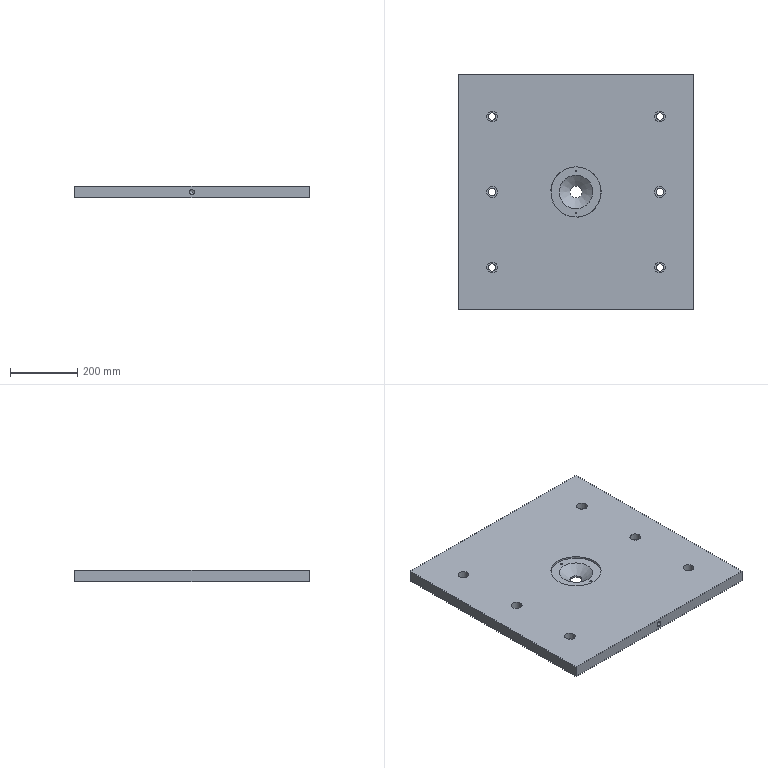Part | NX | features 模具.stp<1>[12] 2 | 1 solid | 55 faces | box 700 x 700 x 35 mm | volume 16813560 mm3 | plane 30 | cylinder 22 | cone 3 | commonest cylinder face diameters 22 x6 32 x6 5 x2 14.1 x2 15.7 x2 16 x2
STEP:
#1=CARTESIAN_POINT('',(-239.,-225.,105.5));
#2=VERTEX_POINT('',#1);
#3=CARTESIAN_POINT('',(-250.,-225.,105.5));
#4=DIRECTION('',(0.,0.,1.));
#5=DIRECTION('',(1.,0.,0.));
#6=AXIS2_PLACEMENT_3D('',#3,#4,#5);
#7=CIRCLE('',#6,11.);
#8=EDGE_CURVE('',#2,#2,#7,.T.);
#9=ORIENTED_EDGE('',*,*,#8,.T.);
#10=EDGE_LOOP('',(#9));
#11=FACE_BOUND('',#10,.T.);
#12=CARTESIAN_POINT('',(-239.,0.,105.5));
#13=VERTEX_POINT('',#12);
#14=CARTESIAN_POINT('',(-250.,0.,105.5));
#15=DIRECTION('',(0.,0.,1.));
#16=DIRECTION('',(1.,0.,0.));
#17=AXIS2_PLACEMENT_3D('',#14,#15,#16);
#18=CIRCLE('',#17,11.);
#19=EDGE_CURVE('',#13,#13,#18,.T.);
#20=ORIENTED_EDGE('',*,*,#19,.T.);
#21=EDGE_LOOP('',(#20));
#22=FACE_BOUND('',#21,.T.);
#23=CARTESIAN_POINT('',(-239.,225.,105.5));
#24=VERTEX_POINT('',#23);
#25=CARTESIAN_POINT('',(-250.,225.,105.5));
#26=DIRECTION('',(0.,0.,1.));
#27=DIRECTION('',(1.,0.,0.));
#28=AXIS2_PLACEMENT_3D('',#25,#26,#27);
#29=CIRCLE('',#28,11.);
#30=EDGE_CURVE('',#24,#24,#29,.T.);
#31=ORIENTED_EDGE('',*,*,#30,.T.);
#32=EDGE_LOOP('',(#31));
#33=FACE_BOUND('',#32,.T.);
#34=CARTESIAN_POINT('',(261.,225.,105.5));
#35=VERTEX_POINT('',#34);
#36=CARTESIAN_POINT('',(250.,225.,105.5));
#37=DIRECTION('',(0.,0.,1.));
#38=DIRECTION('',(1.,0.,0.));
#39=AXIS2_PLACEMENT_3D('',#36,#37,#38);
#40=CIRCLE('',#39,11.);
#41=EDGE_CURVE('',#35,#35,#40,.T.);
#42=ORIENTED_EDGE('',*,*,#41,.T.);
#43=EDGE_LOOP('',(#42));
#44=FACE_BOUND('',#43,.T.);
#45=CARTESIAN_POINT('',(261.,0.,105.5));
#46=VERTEX_POINT('',#45);
#47=CARTESIAN_POINT('',(250.,0.,105.5));
#48=DIRECTION('',(0.,0.,1.));
#49=DIRECTION('',(1.,0.,0.));
#50=AXIS2_PLACEMENT_3D('',#47,#48,#49);
#51=CIRCLE('',#50,11.);
#52=EDGE_CURVE('',#46,#46,#51,.T.);
#53=ORIENTED_EDGE('',*,*,#52,.T.);
#54=EDGE_LOOP('',(#53));
#55=FACE_BOUND('',#54,.T.);
#56=CARTESIAN_POINT('',(261.,-225.,105.5));
#57=VERTEX_POINT('',#56);
#58=CARTESIAN_POINT('',(250.,-225.,105.5));
#59=DIRECTION('',(0.,0.,1.));
#60=DIRECTION('',(1.,0.,0.));
#61=AXIS2_PLACEMENT_3D('',#58,#59,#60);
#62=CIRCLE('',#61,11.);
#63=EDGE_CURVE('',#57,#57,#62,.T.);
#64=ORIENTED_EDGE('',*,*,#63,.T.);
#65=EDGE_LOOP('',(#64));
#66=FACE_BOUND('',#65,.T.);
#67=CARTESIAN_POINT('',(350.,-350.,105.5));
#68=VERTEX_POINT('',#67);
#69=CARTESIAN_POINT('',(350.,350.,105.5));
#70=VERTEX_POINT('',#69);
#71=CARTESIAN_POINT('',(350.,0.,105.5));
#72=DIRECTION('',(0.,1.,0.));
#73=VECTOR('',#72,1000.);
#74=LINE('',#71,#73);
#75=EDGE_CURVE('',#68,#70,#74,.T.);
#76=ORIENTED_EDGE('',*,*,#75,.F.);
#77=CARTESIAN_POINT('',(-350.,-350.,105.5));
#78=VERTEX_POINT('',#77);
#79=CARTESIAN_POINT('',(0.,-350.,105.5));
#80=DIRECTION('',(1.,0.,0.));
#81=VECTOR('',#80,1000.);
#82=LINE('',#79,#81);
#83=EDGE_CURVE('',#78,#68,#82,.T.);
#84=ORIENTED_EDGE('',*,*,#83,.F.);
#85=CARTESIAN_POINT('',(-350.,350.,105.5));
#86=VERTEX_POINT('',#85);
#87=CARTESIAN_POINT('',(-350.,0.,105.5));
#88=DIRECTION('',(0.,-1.,0.));
#89=VECTOR('',#88,1000.);
#90=LINE('',#87,#89);
#91=EDGE_CURVE('',#86,#78,#90,.T.);
#92=ORIENTED_EDGE('',*,*,#91,.F.);
#93=CARTESIAN_POINT('',(0.,350.,105.5));
#94=DIRECTION('',(-1.,0.,0.));
#95=VECTOR('',#94,1000.);
#96=LINE('',#93,#95);
#97=EDGE_CURVE('',#70,#86,#96,.T.);
#98=ORIENTED_EDGE('',*,*,#97,.F.);
#99=EDGE_LOOP('',(#76,#84,#92,#98));
#100=FACE_BOUND('',#99,.T.);
#101=CARTESIAN_POINT('',(312.,-319.,105.5));
#102=VERTEX_POINT('',#101);
#103=CARTESIAN_POINT('',(312.,-322.,105.5));
#104=VERTEX_POINT('',#103);
#105=CARTESIAN_POINT('',(312.,-322.,105.5));
#106=DIRECTION('',(0.,-1.,0.));
#107=VECTOR('',#106,1000.);
#108=LINE('',#105,#107);
#109=EDGE_CURVE('',#102,#104,#108,.T.);
#110=ORIENTED_EDGE('',*,*,#109,.T.);
#111=CARTESIAN_POINT('',(322.,-322.,105.5));
#112=VERTEX_POINT('',#111);
#113=CARTESIAN_POINT('',(312.,-322.,105.5));
#114=DIRECTION('',(1.,0.,0.));
#115=VECTOR('',#114,1000.);
#116=LINE('',#113,#115);
#117=EDGE_CURVE('',#104,#112,#116,.T.);
#118=ORIENTED_EDGE('',*,*,#117,.T.);
#119=CARTESIAN_POINT('',(322.,-312.,105.5));
#120=VERTEX_POINT('',#119);
#121=CARTESIAN_POINT('',(322.,-312.,105.5));
#122=DIRECTION('',(0.,1.,0.));
#123=VECTOR('',#122,1000.);
#124=LINE('',#121,#123);
#125=EDGE_CURVE('',#112,#120,#124,.T.);
#126=ORIENTED_EDGE('',*,*,#125,.T.);
#127=CARTESIAN_POINT('',(319.,-312.,105.5));
#128=VERTEX_POINT('',#127);
#129=CARTESIAN_POINT('',(319.,-312.,105.5));
#130=DIRECTION('',(-1.,0.,0.));
#131=VECTOR('',#130,1000.);
#132=LINE('',#129,#131);
#133=EDGE_CURVE('',#120,#128,#132,.T.);
#134=ORIENTED_EDGE('',*,*,#133,.T.);
#135=CARTESIAN_POINT('',(319.,-319.,105.5));
#136=VERTEX_POINT('',#135);
#137=CARTESIAN_POINT('',(319.,-319.,105.5));
#138=DIRECTION('',(0.,-1.,0.));
#139=VECTOR('',#138,1000.);
#140=LINE('',#137,#139);
#141=EDGE_CURVE('',#128,#136,#140,.T.);
#142=ORIENTED_EDGE('',*,*,#141,.T.);
#143=CARTESIAN_POINT('',(312.,-319.,105.5));
#144=DIRECTION('',(-1.,0.,0.));
#145=VECTOR('',#144,1000.);
#146=LINE('',#143,#145);
#147=EDGE_CURVE('',#136,#102,#146,.T.);
#148=ORIENTED_EDGE('',*,*,#147,.T.);
#149=EDGE_LOOP('',(#110,#118,#126,#134,#142,#148));
#150=FACE_BOUND('',#149,.T.);
#151=CARTESIAN_POINT('',(-18.,0.,105.5));
#152=VERTEX_POINT('',#151);
#153=CARTESIAN_POINT('',(0.,0.,105.5));
#154=DIRECTION('',(0.,0.,-1.));
#155=DIRECTION('',(-1.,0.,0.));
#156=AXIS2_PLACEMENT_3D('',#153,#154,#155);
#157=CIRCLE('',#156,18.);
#158=EDGE_CURVE('',#152,#152,#157,.T.);
#159=ORIENTED_EDGE('',*,*,#158,.F.);
#160=EDGE_LOOP('',(#159));
#161=FACE_BOUND('',#160,.T.);
#162=CARTESIAN_POINT('',(0.,0.,105.5));
#163=DIRECTION('',(0.,0.,-1.));
#164=DIRECTION('',(0.,-1.,0.));
#165=AXIS2_PLACEMENT_3D('',#162,#163,#164);
#166=PLANE('',#165);
#167=ADVANCED_FACE('',(#11,#22,#33,#44,#55,#66,#100,#150,#161),#166,.T.);
#168=CARTESIAN_POINT('',(-18.,0.,110.5));
#169=VERTEX_POINT('',#168);
#170=CARTESIAN_POINT('',(0.,0.,110.5));
#171=DIRECTION('',(0.,0.,1.));
#172=DIRECTION('',(-1.,0.,0.));
#173=AXIS2_PLACEMENT_3D('',#170,#171,#172);
#174=CIRCLE('',#173,18.);
#175=EDGE_CURVE('',#169,#169,#174,.T.);
#176=ORIENTED_EDGE('',*,*,#175,.T.);
#177=EDGE_LOOP('',(#176));
#178=FACE_BOUND('',#177,.T.);
#179=ORIENTED_EDGE('',*,*,#158,.T.);
#180=EDGE_LOOP('',(#179));
#181=FACE_BOUND('',#180,.T.);
#182=CARTESIAN_POINT('',(0.,0.,105.));
#183=DIRECTION('',(0.,0.,1.));
#184=DIRECTION('',(1.,0.,0.));
#185=AXIS2_PLACEMENT_3D('',#182,#183,#184);
#186=CYLINDRICAL_SURFACE('',#185,18.);
#187=ADVANCED_FACE('',(#178,#181),#186,.F.);
#188=ORIENTED_EDGE('',*,*,#109,.F.);
#189=CARTESIAN_POINT('',(312.,-319.,105.8));
#190=VERTEX_POINT('',#189);
#191=CARTESIAN_POINT('',(312.,-319.,105.8));
#192=DIRECTION('',(0.,0.,-1.));
#193=VECTOR('',#192,1000.);
#194=LINE('',#191,#193);
#195=EDGE_CURVE('',#190,#102,#194,.T.);
#196=ORIENTED_EDGE('',*,*,#195,.F.);
#197=CARTESIAN_POINT('',(312.,-322.,105.8));
#198=VERTEX_POINT('',#197);
#199=CARTESIAN_POINT('',(312.,-322.,105.8));
#200=DIRECTION('',(0.,-1.,0.));
#201=VECTOR('',#200,1000.);
#202=LINE('',#199,#201);
#203=EDGE_CURVE('',#190,#198,#202,.T.);
#204=ORIENTED_EDGE('',*,*,#203,.T.);
#205=CARTESIAN_POINT('',(312.,-322.,105.8));
#206=DIRECTION('',(0.,0.,-1.));
#207=VECTOR('',#206,1000.);
#208=LINE('',#205,#207);
#209=EDGE_CURVE('',#198,#104,#208,.T.);
#210=ORIENTED_EDGE('',*,*,#209,.T.);
#211=EDGE_LOOP('',(#188,#196,#204,#210));
#212=FACE_BOUND('',#211,.T.);
#213=CARTESIAN_POINT('',(312.,-322.,105.8));
#214=DIRECTION('',(1.,0.,0.));
#215=DIRECTION('',(0.,1.,0.));
#216=AXIS2_PLACEMENT_3D('',#213,#214,#215);
#217=PLANE('',#216);
#218=ADVANCED_FACE('',(#212),#217,.T.);
#219=ORIENTED_EDGE('',*,*,#117,.F.);
#220=ORIENTED_EDGE('',*,*,#209,.F.);
#221=CARTESIAN_POINT('',(322.,-322.,105.8));
#222=VERTEX_POINT('',#221);
#223=CARTESIAN_POINT('',(312.,-322.,105.8));
#224=DIRECTION('',(1.,0.,0.));
#225=VECTOR('',#224,1000.);
#226=LINE('',#223,#225);
#227=EDGE_CURVE('',#198,#222,#226,.T.);
#228=ORIENTED_EDGE('',*,*,#227,.T.);
#229=CARTESIAN_POINT('',(322.,-322.,105.8));
#230=DIRECTION('',(0.,0.,-1.));
#231=VECTOR('',#230,1000.);
#232=LINE('',#229,#231);
#233=EDGE_CURVE('',#222,#112,#232,.T.);
#234=ORIENTED_EDGE('',*,*,#233,.T.);
#235=EDGE_LOOP('',(#219,#220,#228,#234));
#236=FACE_BOUND('',#235,.T.);
#237=CARTESIAN_POINT('',(312.,-322.,105.8));
#238=DIRECTION('',(0.,1.,0.));
#239=DIRECTION('',(1.,0.,0.));
#240=AXIS2_PLACEMENT_3D('',#237,#238,#239);
#241=PLANE('',#240);
#242=ADVANCED_FACE('',(#236),#241,.T.);
#243=ORIENTED_EDGE('',*,*,#125,.F.);
#244=ORIENTED_EDGE('',*,*,#233,.F.);
#245=CARTESIAN_POINT('',(322.,-312.,105.8));
#246=VERTEX_POINT('',#245);
#247=CARTESIAN_POINT('',(322.,-312.,105.8));
#248=DIRECTION('',(0.,1.,0.));
#249=VECTOR('',#248,1000.);
#250=LINE('',#247,#249);
#251=EDGE_CURVE('',#222,#246,#250,.T.);
#252=ORIENTED_EDGE('',*,*,#251,.T.);
#253=CARTESIAN_POINT('',(322.,-312.,105.8));
#254=DIRECTION('',(0.,0.,-1.));
#255=VECTOR('',#254,1000.);
#256=LINE('',#253,#255);
#257=EDGE_CURVE('',#246,#120,#256,.T.);
#258=ORIENTED_EDGE('',*,*,#257,.T.);
#259=EDGE_LOOP('',(#243,#244,#252,#258));
#260=FACE_BOUND('',#259,.T.);
#261=CARTESIAN_POINT('',(322.,-312.,105.8));
#262=DIRECTION('',(-1.,0.,0.));
#263=DIRECTION('',(0.,0.,1.));
#264=AXIS2_PLACEMENT_3D('',#261,#262,#263);
#265=PLANE('',#264);
#266=ADVANCED_FACE('',(#260),#265,.T.);
#267=ORIENTED_EDGE('',*,*,#133,.F.);
#268=ORIENTED_EDGE('',*,*,#257,.F.);
#269=CARTESIAN_POINT('',(319.,-312.,105.8));
#270=VERTEX_POINT('',#269);
#271=CARTESIAN_POINT('',(319.,-312.,105.8));
#272=DIRECTION('',(-1.,0.,0.));
#273=VECTOR('',#272,1000.);
#274=LINE('',#271,#273);
#275=EDGE_CURVE('',#246,#270,#274,.T.);
#276=ORIENTED_EDGE('',*,*,#275,.T.);
#277=CARTESIAN_POINT('',(319.,-312.,105.8));
#278=DIRECTION('',(0.,0.,-1.));
#279=VECTOR('',#278,1000.);
#280=LINE('',#277,#279);
#281=EDGE_CURVE('',#270,#128,#280,.T.);
#282=ORIENTED_EDGE('',*,*,#281,.T.);
#283=EDGE_LOOP('',(#267,#268,#276,#282));
#284=FACE_BOUND('',#283,.T.);
#285=CARTESIAN_POINT('',(319.,-312.,105.8));
#286=DIRECTION('',(0.,-1.,0.));
#287=DIRECTION('',(0.,0.,-1.));
#288=AXIS2_PLACEMENT_3D('',#285,#286,#287);
#289=PLANE('',#288);
#290=ADVANCED_FACE('',(#284),#289,.T.);
#291=ORIENTED_EDGE('',*,*,#141,.F.);
#292=ORIENTED_EDGE('',*,*,#281,.F.);
#293=CARTESIAN_POINT('',(319.,-319.,105.8));
#294=VERTEX_POINT('',#293);
#295=CARTESIAN_POINT('',(319.,-319.,105.8));
#296=DIRECTION('',(0.,-1.,0.));
#297=VECTOR('',#296,1000.);
#298=LINE('',#295,#297);
#299=EDGE_CURVE('',#270,#294,#298,.T.);
#300=ORIENTED_EDGE('',*,*,#299,.T.);
#301=CARTESIAN_POINT('',(319.,-319.,105.8));
#302=DIRECTION('',(0.,0.,-1.));
#303=VECTOR('',#302,1000.);
#304=LINE('',#301,#303);
#305=EDGE_CURVE('',#294,#136,#304,.T.);
#306=ORIENTED_EDGE('',*,*,#305,.T.);
#307=EDGE_LOOP('',(#291,#292,#300,#306));
#308=FACE_BOUND('',#307,.T.);
#309=CARTESIAN_POINT('',(319.,-319.,105.8));
#310=DIRECTION('',(1.,0.,0.));
#311=DIRECTION('',(0.,1.,0.));
#312=AXIS2_PLACEMENT_3D('',#309,#310,#311);
#313=PLANE('',#312);
#314=ADVANCED_FACE('',(#308),#313,.T.);
#315=ORIENTED_EDGE('',*,*,#147,.F.);
#316=ORIENTED_EDGE('',*,*,#305,.F.);
#317=CARTESIAN_POINT('',(312.,-319.,105.8));
#318=DIRECTION('',(-1.,0.,0.));
#319=VECTOR('',#318,1000.);
#320=LINE('',#317,#319);
#321=EDGE_CURVE('',#294,#190,#320,.T.);
#322=ORIENTED_EDGE('',*,*,#321,.T.);
#323=ORIENTED_EDGE('',*,*,#195,.T.);
#324=EDGE_LOOP('',(#315,#316,#322,#323));
#325=FACE_BOUND('',#324,.T.);
#326=CARTESIAN_POINT('',(312.,-319.,105.8));
#327=DIRECTION('',(0.,-1.,0.));
#328=DIRECTION('',(0.,0.,-1.));
#329=AXIS2_PLACEMENT_3D('',#326,#327,#328);
#330=PLANE('',#329);
#331=ADVANCED_FACE('',(#325),#330,.T.);
#332=ORIENTED_EDGE('',*,*,#227,.F.);
#333=ORIENTED_EDGE('',*,*,#203,.F.);
#334=ORIENTED_EDGE('',*,*,#321,.F.);
#335=ORIENTED_EDGE('',*,*,#299,.F.);
#336=ORIENTED_EDGE('',*,*,#275,.F.);
#337=ORIENTED_EDGE('',*,*,#251,.F.);
#338=EDGE_LOOP('',(#332,#333,#334,#335,#336,#337));
#339=FACE_BOUND('',#338,.T.);
#340=CARTESIAN_POINT('',(322.,-322.,105.8));
#341=DIRECTION('',(0.,0.,1.));
#342=DIRECTION('',(1.,0.,0.));
#343=AXIS2_PLACEMENT_3D('',#340,#341,#342);
#344=PLANE('',#343);
#345=ADVANCED_FACE('',(#339),#344,.F.);
#346=CARTESIAN_POINT('',(0.,65.,122.5));
#347=VERTEX_POINT('',#346);
#348=CARTESIAN_POINT('',(0.,62.5,122.5));
#349=DIRECTION('',(0.,0.,-1.));
#350=DIRECTION('',(0.,1.,0.));
#351=AXIS2_PLACEMENT_3D('',#348,#349,#350);
#352=CIRCLE('',#351,2.5);
#353=EDGE_CURVE('',#347,#347,#352,.T.);
#354=ORIENTED_EDGE('',*,*,#353,.F.);
#355=EDGE_LOOP('',(#354));
#356=FACE_BOUND('',#355,.T.);
#357=CARTESIAN_POINT('',(0.,62.5,122.5));
#358=DIRECTION('',(0.,0.,-1.));
#359=DIRECTION('',(-1.,0.,0.));
#360=AXIS2_PLACEMENT_3D('',#357,#358,#359);
#361=PLANE('',#360);
#362=ADVANCED_FACE('',(#356),#361,.F.);
#363=CARTESIAN_POINT('',(0.,65.,135.5));
#364=VERTEX_POINT('',#363);
#365=CARTESIAN_POINT('',(0.,62.5,135.5));
#366=DIRECTION('',(0.,0.,-1.));
#367=DIRECTION('',(0.,1.,0.));
#368=AXIS2_PLACEMENT_3D('',#365,#366,#367);
#369=CIRCLE('',#368,2.5);
#370=EDGE_CURVE('',#364,#364,#369,.T.);
#371=ORIENTED_EDGE('',*,*,#370,.F.);
#372=EDGE_LOOP('',(#371));
#373=FACE_BOUND('',#372,.T.);
#374=ORIENTED_EDGE('',*,*,#353,.T.);
#375=EDGE_LOOP('',(#374));
#376=FACE_BOUND('',#375,.T.);
#377=CARTESIAN_POINT('',(0.,62.5,127.5));
#378=DIRECTION('',(0.,0.,1.));
#379=DIRECTION('',(1.,0.,0.));
#380=AXIS2_PLACEMENT_3D('',#377,#378,#379);
#381=CYLINDRICAL_SURFACE('',#380,2.5);
#382=ADVANCED_FACE('',(#373,#376),#381,.F.);
#383=CARTESIAN_POINT('',(0.,-60.,122.5));
#384=VERTEX_POINT('',#383);
#385=CARTESIAN_POINT('',(0.,-62.5,122.5));
#386=DIRECTION('',(0.,0.,-1.));
#387=DIRECTION('',(0.,1.,0.));
#388=AXIS2_PLACEMENT_3D('',#385,#386,#387);
#389=CIRCLE('',#388,2.5);
#390=EDGE_CURVE('',#384,#384,#389,.T.);
#391=ORIENTED_EDGE('',*,*,#390,.F.);
#392=EDGE_LOOP('',(#391));
#393=FACE_BOUND('',#392,.T.);
#394=CARTESIAN_POINT('',(0.,-62.5,122.5));
#395=DIRECTION('',(0.,0.,-1.));
#396=DIRECTION('',(-1.,0.,0.));
#397=AXIS2_PLACEMENT_3D('',#394,#395,#396);
#398=PLANE('',#397);
#399=ADVANCED_FACE('',(#393),#398,.F.);
#400=CARTESIAN_POINT('',(0.,-60.,135.5));
#401=VERTEX_POINT('',#400);
#402=CARTESIAN_POINT('',(0.,-62.5,135.5));
#403=DIRECTION('',(0.,0.,-1.));
#404=DIRECTION('',(0.,1.,0.));
#405=AXIS2_PLACEMENT_3D('',#402,#403,#404);
#406=CIRCLE('',#405,2.5);
#407=EDGE_CURVE('',#401,#401,#406,.T.);
#408=ORIENTED_EDGE('',*,*,#407,.F.);
#409=EDGE_LOOP('',(#408));
#410=FACE_BOUND('',#409,.T.);
#411=ORIENTED_EDGE('',*,*,#390,.T.);
#412=EDGE_LOOP('',(#411));
#413=FACE_BOUND('',#412,.T.);
#414=CARTESIAN_POINT('',(0.,-62.5,127.5));
#415=DIRECTION('',(0.,0.,1.));
#416=DIRECTION('',(1.,0.,0.));
#417=AXIS2_PLACEMENT_3D('',#414,#415,#416);
#418=CYLINDRICAL_SURFACE('',#417,2.5);
#419=ADVANCED_FACE('',(#410,#413),#418,.F.);
#420=CARTESIAN_POINT('',(0.,75.,135.5));
#421=VERTEX_POINT('',#420);
#422=CARTESIAN_POINT('',(0.,0.,135.5));
#423=DIRECTION('',(0.,0.,-1.));
#424=DIRECTION('',(0.,1.,0.));
#425=AXIS2_PLACEMENT_3D('',#422,#423,#424);
#426=CIRCLE('',#425,75.);
#427=EDGE_CURVE('',#421,#421,#426,.T.);
#428=ORIENTED_EDGE('',*,*,#427,.T.);
#429=EDGE_LOOP('',(#428));
#430=FACE_BOUND('',#429,.T.);
#431=CARTESIAN_POINT('',(75.,0.,140.5));
#432=VERTEX_POINT('',#431);
#433=CARTESIAN_POINT('',(0.,0.,140.5));
#434=DIRECTION('',(0.,0.,1.));
#435=DIRECTION('',(1.,0.,0.));
#436=AXIS2_PLACEMENT_3D('',#433,#434,#435);
#437=CIRCLE('',#436,75.);
#438=EDGE_CURVE('',#432,#432,#437,.T.);
#439=ORIENTED_EDGE('',*,*,#438,.T.);
#440=EDGE_LOOP('',(#439));
#441=FACE_BOUND('',#440,.T.);
#442=CARTESIAN_POINT('',(0.,0.,150.5));
#443=DIRECTION('',(0.,0.,-1.));
#444=DIRECTION('',(0.,1.,0.));
#445=AXIS2_PLACEMENT_3D('',#442,#443,#444);
#446=CYLINDRICAL_SURFACE('',#445,75.);
#447=ADVANCED_FACE('',(#430,#441),#446,.F.);
#448=CARTESIAN_POINT('',(0.,49.999,135.5));
#449=VERTEX_POINT('',#448);
#450=CARTESIAN_POINT('',(0.,0.,135.5));
#451=DIRECTION('',(0.,0.,1.));
#452=DIRECTION('',(0.,1.,0.));
#453=AXIS2_PLACEMENT_3D('',#450,#451,#452);
#454=CIRCLE('',#453,49.999);
#455=EDGE_CURVE('',#449,#449,#454,.T.);
#456=ORIENTED_EDGE('',*,*,#455,.F.);
#457=EDGE_LOOP('',(#456));
#458=FACE_BOUND('',#457,.T.);
#459=ORIENTED_EDGE('',*,*,#427,.F.);
#460=EDGE_LOOP('',(#459));
#461=FACE_BOUND('',#460,.T.);
#462=ORIENTED_EDGE('',*,*,#407,.T.);
#463=EDGE_LOOP('',(#462));
#464=FACE_BOUND('',#463,.T.);
#465=ORIENTED_EDGE('',*,*,#370,.T.);
#466=EDGE_LOOP('',(#465));
#467=FACE_BOUND('',#466,.T.);
#468=CARTESIAN_POINT('',(0.,0.,135.5));
#469=DIRECTION('',(0.,0.,-1.));
#470=DIRECTION('',(-1.,0.,0.));
#471=AXIS2_PLACEMENT_3D('',#468,#469,#470);
#472=PLANE('',#471);
#473=ADVANCED_FACE('',(#458,#461,#464,#467),#472,.F.);
#474=CARTESIAN_POINT('',(-234.,-225.,119.5));
#475=VERTEX_POINT('',#474);
#476=CARTESIAN_POINT('',(-250.,-225.,119.5));
#477=DIRECTION('',(0.,0.,1.));
#478=DIRECTION('',(1.,0.,0.));
#479=AXIS2_PLACEMENT_3D('',#476,#477,#478);
#480=CIRCLE('',#479,16.);
#481=EDGE_CURVE('',#475,#475,#480,.T.);
#482=ORIENTED_EDGE('',*,*,#481,.F.);
#483=EDGE_LOOP('',(#482));
#484=FACE_BOUND('',#483,.T.);
#485=CARTESIAN_POINT('',(-234.,-225.,140.5));
#486=VERTEX_POINT('',#485);
#487=CARTESIAN_POINT('',(-250.,-225.,140.5));
#488=DIRECTION('',(0.,0.,-1.));
#489=DIRECTION('',(1.,0.,0.));
#490=AXIS2_PLACEMENT_3D('',#487,#488,#489);
#491=CIRCLE('',#490,16.);
#492=EDGE_CURVE('',#486,#486,#491,.T.);
#493=ORIENTED_EDGE('',*,*,#492,.F.);
#494=EDGE_LOOP('',(#493));
#495=FACE_BOUND('',#494,.T.);
#496=CARTESIAN_POINT('',(-250.,-225.,119.5));
#497=DIRECTION('',(0.,0.,1.));
#498=DIRECTION('',(1.,0.,0.));
#499=AXIS2_PLACEMENT_3D('',#496,#497,#498);
#500=CYLINDRICAL_SURFACE('',#499,16.);
#501=ADVANCED_FACE('',(#484,#495),#500,.F.);
#502=ORIENTED_EDGE('',*,*,#481,.T.);
#503=EDGE_LOOP('',(#502));
#504=FACE_BOUND('',#503,.T.);
#505=CARTESIAN_POINT('',(-261.,-225.,119.5));
#506=VERTEX_POINT('',#505);
#507=CARTESIAN_POINT('',(-250.,-225.,119.5));
#508=DIRECTION('',(0.,0.,1.));
#509=DIRECTION('',(-1.,0.,0.));
#510=AXIS2_PLACEMENT_3D('',#507,#508,#509);
#511=CIRCLE('',#510,11.);
#512=EDGE_CURVE('',#506,#506,#511,.T.);
#513=ORIENTED_EDGE('',*,*,#512,.F.);
#514=EDGE_LOOP('',(#513));
#515=FACE_BOUND('',#514,.T.);
#516=CARTESIAN_POINT('',(-250.,-225.,119.5));
#517=DIRECTION('',(0.,0.,-1.));
#518=DIRECTION('',(0.,-1.,0.));
#519=AXIS2_PLACEMENT_3D('',#516,#517,#518);
#520=PLANE('',#519);
#521=ADVANCED_FACE('',(#504,#515),#520,.F.);
#522=CARTESIAN_POINT('',(-234.,0.,119.5));
#523=VERTEX_POINT('',#522);
#524=CARTESIAN_POINT('',(-250.,0.,119.5));
#525=DIRECTION('',(0.,0.,1.));
#526=DIRECTION('',(1.,0.,0.));
#527=AXIS2_PLACEMENT_3D('',#524,#525,#526);
#528=CIRCLE('',#527,16.);
#529=EDGE_CURVE('',#523,#523,#528,.T.);
#530=ORIENTED_EDGE('',*,*,#529,.F.);
#531=EDGE_LOOP('',(#530));
#532=FACE_BOUND('',#531,.T.);
#533=CARTESIAN_POINT('',(-234.,0.,140.5));
#534=VERTEX_POINT('',#533);
#535=CARTESIAN_POINT('',(-250.,0.,140.5));
#536=DIRECTION('',(0.,0.,-1.));
#537=DIRECTION('',(1.,0.,0.));
#538=AXIS2_PLACEMENT_3D('',#535,#536,#537);
#539=CIRCLE('',#538,16.);
#540=EDGE_CURVE('',#534,#534,#539,.T.);
#541=ORIENTED_EDGE('',*,*,#540,.F.);
#542=EDGE_LOOP('',(#541));
#543=FACE_BOUND('',#542,.T.);
#544=CARTESIAN_POINT('',(-250.,0.,119.5));
#545=DIRECTION('',(0.,0.,1.));
#546=DIRECTION('',(1.,0.,0.));
#547=AXIS2_PLACEMENT_3D('',#544,#545,#546);
#548=CYLINDRICAL_SURFACE('',#547,16.);
#549=ADVANCED_FACE('',(#532,#543),#548,.F.);
#550=ORIENTED_EDGE('',*,*,#529,.T.);
#551=EDGE_LOOP('',(#550));
#552=FACE_BOUND('',#551,.T.);
#553=CARTESIAN_POINT('',(-261.,0.,119.5));
#554=VERTEX_POINT('',#553);
#555=CARTESIAN_POINT('',(-250.,0.,119.5));
#556=DIRECTION('',(0.,0.,1.));
#557=DIRECTION('',(-1.,0.,0.));
#558=AXIS2_PLACEMENT_3D('',#555,#556,#557);
#559=CIRCLE('',#558,11.);
#560=EDGE_CURVE('',#554,#554,#559,.T.);
#561=ORIENTED_EDGE('',*,*,#560,.F.);
#562=EDGE_LOOP('',(#561));
#563=FACE_BOUND('',#562,.T.);
#564=CARTESIAN_POINT('',(-250.,0.,119.5));
#565=DIRECTION('',(0.,0.,-1.));
#566=DIRECTION('',(0.,-1.,0.));
#567=AXIS2_PLACEMENT_3D('',#564,#565,#566);
#568=PLANE('',#567);
#569=ADVANCED_FACE('',(#552,#563),#568,.F.);
#570=CARTESIAN_POINT('',(-234.,225.,119.5));
#571=VERTEX_POINT('',#570);
#572=CARTESIAN_POINT('',(-250.,225.,119.5));
#573=DIRECTION('',(0.,0.,1.));
#574=DIRECTION('',(1.,0.,0.));
#575=AXIS2_PLACEMENT_3D('',#572,#573,#574);
#576=CIRCLE('',#575,16.);
#577=EDGE_CURVE('',#571,#571,#576,.T.);
#578=ORIENTED_EDGE('',*,*,#577,.F.);
#579=EDGE_LOOP('',(#578));
#580=FACE_BOUND('',#579,.T.);
#581=CARTESIAN_POINT('',(-234.,225.,140.5));
#582=VERTEX_POINT('',#581);
#583=CARTESIAN_POINT('',(-250.,225.,140.5));
#584=DIRECTION('',(0.,0.,-1.));
#585=DIRECTION('',(1.,0.,0.));
#586=AXIS2_PLACEMENT_3D('',#583,#584,#585);
#587=CIRCLE('',#586,16.);
#588=EDGE_CURVE('',#582,#582,#587,.T.);
#589=ORIENTED_EDGE('',*,*,#588,.F.);
#590=EDGE_LOOP('',(#589));
#591=FACE_BOUND('',#590,.T.);
#592=CARTESIAN_POINT('',(-250.,225.,119.5));
#593=DIRECTION('',(0.,0.,1.));
#594=DIRECTION('',(1.,0.,0.));
#595=AXIS2_PLACEMENT_3D('',#592,#593,#594);
#596=CYLINDRICAL_SURFACE('',#595,16.);
#597=ADVANCED_FACE('',(#580,#591),#596,.F.);
#598=ORIENTED_EDGE('',*,*,#577,.T.);
#599=EDGE_LOOP('',(#598));
#600=FACE_BOUND('',#599,.T.);
#601=CARTESIAN_POINT('',(-261.,225.,119.5));
#602=VERTEX_POINT('',#601);
#603=CARTESIAN_POINT('',(-250.,225.,119.5));
#604=DIRECTION('',(0.,0.,1.));
#605=DIRECTION('',(-1.,0.,0.));
#606=AXIS2_PLACEMENT_3D('',#603,#604,#605);
#607=CIRCLE('',#606,11.);
#608=EDGE_CURVE('',#602,#602,#607,.T.);
#609=ORIENTED_EDGE('',*,*,#608,.F.);
#610=EDGE_LOOP('',(#609));
#611=FACE_BOUND('',#610,.T.);
#612=CARTESIAN_POINT('',(-250.,225.,119.5));
#613=DIRECTION('',(0.,0.,-1.));
#614=DIRECTION('',(0.,-1.,0.));
#615=AXIS2_PLACEMENT_3D('',#612,#613,#614);
#616=PLANE('',#615);
#617=ADVANCED_FACE('',(#600,#611),#616,.F.);
#618=CARTESIAN_POINT('',(266.,225.,119.5));
#619=VERTEX_POINT('',#618);
#620=CARTESIAN_POINT('',(250.,225.,119.5));
#621=DIRECTION('',(0.,0.,1.));
#622=DIRECTION('',(1.,0.,0.));
#623=AXIS2_PLACEMENT_3D('',#620,#621,#622);
#624=CIRCLE('',#623,16.);
#625=EDGE_CURVE('',#619,#619,#624,.T.);
#626=ORIENTED_EDGE('',*,*,#625,.F.);
#627=EDGE_LOOP('',(#626));
#628=FACE_BOUND('',#627,.T.);
#629=CARTESIAN_POINT('',(266.,225.,140.5));
#630=VERTEX_POINT('',#629);
#631=CARTESIAN_POINT('',(250.,225.,140.5));
#632=DIRECTION('',(0.,0.,-1.));
#633=DIRECTION('',(1.,0.,0.));
#634=AXIS2_PLACEMENT_3D('',#631,#632,#633);
#635=CIRCLE('',#634,16.);
#636=EDGE_CURVE('',#630,#630,#635,.T.);
#637=ORIENTED_EDGE('',*,*,#636,.F.);
#638=EDGE_LOOP('',(#637));
#639=FACE_BOUND('',#638,.T.);
#640=CARTESIAN_POINT('',(250.,225.,119.5));
#641=DIRECTION('',(0.,0.,1.));
#642=DIRECTION('',(1.,0.,0.));
#643=AXIS2_PLACEMENT_3D('',#640,#641,#642);
#644=CYLINDRICAL_SURFACE('',#643,16.);
#645=ADVANCED_FACE('',(#628,#639),#644,.F.);
#646=ORIENTED_EDGE('',*,*,#625,.T.);
#647=EDGE_LOOP('',(#646));
#648=FACE_BOUND('',#647,.T.);
#649=CARTESIAN_POINT('',(239.,225.,119.5));
#650=VERTEX_POINT('',#649);
#651=CARTESIAN_POINT('',(250.,225.,119.5));
#652=DIRECTION('',(0.,0.,1.));
#653=DIRECTION('',(-1.,0.,0.));
#654=AXIS2_PLACEMENT_3D('',#651,#652,#653);
#655=CIRCLE('',#654,11.);
#656=EDGE_CURVE('',#650,#650,#655,.T.);
#657=ORIENTED_EDGE('',*,*,#656,.F.);
#658=EDGE_LOOP('',(#657));
#659=FACE_BOUND('',#658,.T.);
#660=CARTESIAN_POINT('',(250.,225.,119.5));
#661=DIRECTION('',(0.,0.,-1.));
#662=DIRECTION('',(0.,-1.,0.));
#663=AXIS2_PLACEMENT_3D('',#660,#661,#662);
#664=PLANE('',#663);
#665=ADVANCED_FACE('',(#648,#659),#664,.F.);
#666=CARTESIAN_POINT('',(266.,0.,119.5));
#667=VERTEX_POINT('',#666);
#668=CARTESIAN_POINT('',(250.,0.,119.5));
#669=DIRECTION('',(0.,0.,1.));
#670=DIRECTION('',(1.,0.,0.));
#671=AXIS2_PLACEMENT_3D('',#668,#669,#670);
#672=CIRCLE('',#671,16.);
#673=EDGE_CURVE('',#667,#667,#672,.T.);
#674=ORIENTED_EDGE('',*,*,#673,.F.);
#675=EDGE_LOOP('',(#674));
#676=FACE_BOUND('',#675,.T.);
#677=CARTESIAN_POINT('',(266.,0.,140.5));
#678=VERTEX_POINT('',#677);
#679=CARTESIAN_POINT('',(250.,0.,140.5));
#680=DIRECTION('',(0.,0.,-1.));
#681=DIRECTION('',(1.,0.,0.));
#682=AXIS2_PLACEMENT_3D('',#679,#680,#681);
#683=CIRCLE('',#682,16.);
#684=EDGE_CURVE('',#678,#678,#683,.T.);
#685=ORIENTED_EDGE('',*,*,#684,.F.);
#686=EDGE_LOOP('',(#685));
#687=FACE_BOUND('',#686,.T.);
#688=CARTESIAN_POINT('',(250.,0.,119.5));
#689=DIRECTION('',(0.,0.,1.));
#690=DIRECTION('',(1.,0.,0.));
#691=AXIS2_PLACEMENT_3D('',#688,#689,#690);
#692=CYLINDRICAL_SURFACE('',#691,16.);
#693=ADVANCED_FACE('',(#676,#687),#692,.F.);
#694=ORIENTED_EDGE('',*,*,#673,.T.);
#695=EDGE_LOOP('',(#694));
#696=FACE_BOUND('',#695,.T.);
#697=CARTESIAN_POINT('',(239.,0.,119.5));
#698=VERTEX_POINT('',#697);
#699=CARTESIAN_POINT('',(250.,0.,119.5));
#700=DIRECTION('',(0.,0.,1.));
#701=DIRECTION('',(-1.,0.,0.));
#702=AXIS2_PLACEMENT_3D('',#699,#700,#701);
#703=CIRCLE('',#702,11.);
#704=EDGE_CURVE('',#698,#698,#703,.T.);
#705=ORIENTED_EDGE('',*,*,#704,.F.);
#706=EDGE_LOOP('',(#705));
#707=FACE_BOUND('',#706,.T.);
#708=CARTESIAN_POINT('',(250.,0.,119.5));
#709=DIRECTION('',(0.,0.,-1.));
#710=DIRECTION('',(0.,-1.,0.));
#711=AXIS2_PLACEMENT_3D('',#708,#709,#710);
#712=PLANE('',#711);
#713=ADVANCED_FACE('',(#696,#707),#712,.F.);
#714=CARTESIAN_POINT('',(266.,-225.,119.5));
#715=VERTEX_POINT('',#714);
#716=CARTESIAN_POINT('',(250.,-225.,119.5));
#717=DIRECTION('',(0.,0.,1.));
#718=DIRECTION('',(1.,0.,0.));
#719=AXIS2_PLACEMENT_3D('',#716,#717,#718);
#720=CIRCLE('',#719,16.);
#721=EDGE_CURVE('',#715,#715,#720,.T.);
#722=ORIENTED_EDGE('',*,*,#721,.F.);
#723=EDGE_LOOP('',(#722));
#724=FACE_BOUND('',#723,.T.);
#725=CARTESIAN_POINT('',(266.,-225.,140.5));
#726=VERTEX_POINT('',#725);
#727=CARTESIAN_POINT('',(250.,-225.,140.5));
#728=DIRECTION('',(0.,0.,-1.));
#729=DIRECTION('',(1.,0.,0.));
#730=AXIS2_PLACEMENT_3D('',#727,#728,#729);
#731=CIRCLE('',#730,16.);
#732=EDGE_CURVE('',#726,#726,#731,.T.);
#733=ORIENTED_EDGE('',*,*,#732,.F.);
#734=EDGE_LOOP('',(#733));
#735=FACE_BOUND('',#734,.T.);
#736=CARTESIAN_POINT('',(250.,-225.,119.5));
#737=DIRECTION('',(0.,0.,1.));
#738=DIRECTION('',(1.,0.,0.));
#739=AXIS2_PLACEMENT_3D('',#736,#737,#738);
#740=CYLINDRICAL_SURFACE('',#739,16.);
#741=ADVANCED_FACE('',(#724,#735),#740,.F.);
#742=ORIENTED_EDGE('',*,*,#721,.T.);
#743=EDGE_LOOP('',(#742));
#744=FACE_BOUND('',#743,.T.);
#745=CARTESIAN_POINT('',(239.,-225.,119.5));
#746=VERTEX_POINT('',#745);
#747=CARTESIAN_POINT('',(250.,-225.,119.5));
#748=DIRECTION('',(0.,0.,1.));
#749=DIRECTION('',(-1.,0.,0.));
#750=AXIS2_PLACEMENT_3D('',#747,#748,#749);
#751=CIRCLE('',#750,11.);
#752=EDGE_CURVE('',#746,#746,#751,.T.);
#753=ORIENTED_EDGE('',*,*,#752,.F.);
#754=EDGE_LOOP('',(#753));
#755=FACE_BOUND('',#754,.T.);
#756=CARTESIAN_POINT('',(250.,-225.,119.5));
#757=DIRECTION('',(0.,0.,-1.));
#758=DIRECTION('',(0.,-1.,0.));
#759=AXIS2_PLACEMENT_3D('',#756,#757,#758);
#760=PLANE('',#759);
#761=ADVANCED_FACE('',(#744,#755),#760,.F.);
#762=CARTESIAN_POINT('',(0.,-311.005,123.));
#763=VERTEX_POINT('',#762);
#764=VERTEX_LOOP('',#763);
#765=FACE_BOUND('',#764,.T.);
#766=CARTESIAN_POINT('',(7.05,-315.075,123.));
#767=VERTEX_POINT('',#766);
#768=CARTESIAN_POINT('',(0.,-315.075,123.));
#769=DIRECTION('',(0.,1.,0.));
#770=DIRECTION('',(1.,0.,0.));
#771=AXIS2_PLACEMENT_3D('',#768,#769,#770);
#772=CIRCLE('',#771,7.05);
#773=EDGE_CURVE('',#767,#767,#772,.T.);
#774=ORIENTED_EDGE('',*,*,#773,.F.);
#775=EDGE_LOOP('',(#774));
#776=FACE_BOUND('',#775,.T.);
#777=CARTESIAN_POINT('',(0.,-312.005,123.));
#778=DIRECTION('',(0.,-1.,0.));
#779=DIRECTION('',(1.,0.,0.));
#780=AXIS2_PLACEMENT_3D('',#777,#778,#779);
#781=CONICAL_SURFACE('',#780,1.732,1.047);
#782=ADVANCED_FACE('',(#765,#776),#781,.F.);
#783=CARTESIAN_POINT('',(7.05,-321.,123.));
#784=VERTEX_POINT('',#783);
#785=CARTESIAN_POINT('',(7.05,-322.,123.));
#786=VERTEX_POINT('',#785);
#787=CARTESIAN_POINT('',(7.05,-315.075,123.));
#788=DIRECTION('',(0.,-1.,0.));
#789=VECTOR('',#788,1000.);
#790=LINE('',#787,#789);
#791=EDGE_CURVE('',#784,#786,#790,.T.);
#792=ORIENTED_EDGE('',*,*,#791,.T.);
#793=CARTESIAN_POINT('',(0.,-322.,130.05));
#794=VERTEX_POINT('',#793);
#795=CARTESIAN_POINT('',(0.,-322.,123.));
#796=DIRECTION('',(0.,1.,0.));
#797=DIRECTION('',(0.,0.,1.));
#798=AXIS2_PLACEMENT_3D('',#795,#796,#797);
#799=CIRCLE('',#798,7.05);
#800=EDGE_CURVE('',#786,#794,#799,.T.);
#801=ORIENTED_EDGE('',*,*,#800,.T.);
#802=CARTESIAN_POINT('',(0.,-321.,130.05));
#803=VERTEX_POINT('',#802);
#804=CARTESIAN_POINT('',(0.,-315.075,130.05));
#805=DIRECTION('',(0.,1.,0.));
#806=VECTOR('',#805,1000.);
#807=LINE('',#804,#806);
#808=EDGE_CURVE('',#794,#803,#807,.T.);
#809=ORIENTED_EDGE('',*,*,#808,.T.);
#810=CARTESIAN_POINT('',(0.,-321.,123.));
#811=DIRECTION('',(0.,1.,0.));
#812=DIRECTION('',(0.,0.,1.));
#813=AXIS2_PLACEMENT_3D('',#810,#811,#812);
#814=CIRCLE('',#813,7.05);
#815=EDGE_CURVE('',#784,#803,#814,.T.);
#816=ORIENTED_EDGE('',*,*,#815,.F.);
#817=EDGE_LOOP('',(#792,#801,#809,#816));
#818=FACE_BOUND('',#817,.T.);
#819=ORIENTED_EDGE('',*,*,#773,.T.);
#820=EDGE_LOOP('',(#819));
#821=FACE_BOUND('',#820,.T.);
#822=CARTESIAN_POINT('',(0.,-350.,115.95));
#823=VERTEX_POINT('',#822);
#824=CARTESIAN_POINT('',(0.,-350.,123.));
#825=DIRECTION('',(0.,-1.,0.));
#826=DIRECTION('',(0.,0.,-1.));
#827=AXIS2_PLACEMENT_3D('',#824,#825,#826);
#828=CIRCLE('',#827,7.05);
#829=EDGE_CURVE('',#823,#823,#828,.T.);
#830=ORIENTED_EDGE('',*,*,#829,.T.);
#831=EDGE_LOOP('',(#830));
#832=FACE_BOUND('',#831,.T.);
#833=CARTESIAN_POINT('',(0.,-315.075,123.));
#834=DIRECTION('',(0.,-1.,0.));
#835=DIRECTION('',(1.,0.,0.));
#836=AXIS2_PLACEMENT_3D('',#833,#834,#835);
#837=CYLINDRICAL_SURFACE('',#836,7.05);
#838=ADVANCED_FACE('',(#818,#821,#832),#837,.F.);
#839=CARTESIAN_POINT('',(0.,-321.,131.));
#840=VERTEX_POINT('',#839);
#841=CARTESIAN_POINT('',(0.,-350.,131.));
#842=VERTEX_POINT('',#841);
#843=CARTESIAN_POINT('',(0.,-321.,131.));
#844=DIRECTION('',(0.,-1.,0.));
#845=VECTOR('',#844,1000.);
#846=LINE('',#843,#845);
#847=EDGE_CURVE('',#840,#842,#846,.T.);
#848=ORIENTED_EDGE('',*,*,#847,.F.);
#849=CARTESIAN_POINT('',(0.,-321.,131.));
#850=DIRECTION('',(0.,0.,-1.));
#851=VECTOR('',#850,1000.);
#852=LINE('',#849,#851);
#853=EDGE_CURVE('',#840,#803,#852,.T.);
#854=ORIENTED_EDGE('',*,*,#853,.T.);
#855=ORIENTED_EDGE('',*,*,#808,.F.);
#856=CARTESIAN_POINT('',(0.,-322.,130.85));
#857=VERTEX_POINT('',#856);
#858=CARTESIAN_POINT('',(0.,-322.,123.));
#859=DIRECTION('',(0.,0.,1.));
#860=VECTOR('',#859,1000.);
#861=LINE('',#858,#860);
#862=EDGE_CURVE('',#794,#857,#861,.T.);
#863=ORIENTED_EDGE('',*,*,#862,.T.);
#864=CARTESIAN_POINT('',(0.,-350.,130.85));
#865=VERTEX_POINT('',#864);
#866=CARTESIAN_POINT('',(0.,-322.,130.85));
#867=DIRECTION('',(0.,-1.,0.));
#868=VECTOR('',#867,1000.);
#869=LINE('',#866,#868);
#870=EDGE_CURVE('',#857,#865,#869,.T.);
#871=ORIENTED_EDGE('',*,*,#870,.T.);
#872=CARTESIAN_POINT('',(0.,-350.,105.5));
#873=DIRECTION('',(0.,0.,-1.));
#874=VECTOR('',#873,1000.);
#875=LINE('',#872,#874);
#876=EDGE_CURVE('',#842,#865,#875,.T.);
#877=ORIENTED_EDGE('',*,*,#876,.F.);
#878=EDGE_LOOP('',(#848,#854,#855,#863,#871,#877));
#879=FACE_BOUND('',#878,.T.);
#880=CARTESIAN_POINT('',(0.,-321.,131.));
#881=DIRECTION('',(-1.,0.,0.));
#882=DIRECTION('',(0.,0.,1.));
#883=AXIS2_PLACEMENT_3D('',#880,#881,#882);
#884=PLANE('',#883);
#885=ADVANCED_FACE('',(#879),#884,.T.);
#886=CARTESIAN_POINT('',(7.85,-350.,123.));
#887=VERTEX_POINT('',#886);
#888=CARTESIAN_POINT('',(7.85,-322.,123.));
#889=VERTEX_POINT('',#888);
#890=CARTESIAN_POINT('',(7.85,-322.,123.));
#891=DIRECTION('',(0.,1.,0.));
#892=VECTOR('',#891,1000.);
#893=LINE('',#890,#892);
#894=EDGE_CURVE('',#887,#889,#893,.T.);
#895=ORIENTED_EDGE('',*,*,#894,.T.);
#896=CARTESIAN_POINT('',(0.,-322.,123.));
#897=DIRECTION('',(-1.,0.,0.));
#898=VECTOR('',#897,1000.);
#899=LINE('',#896,#898);
#900=EDGE_CURVE('',#889,#786,#899,.T.);
#901=ORIENTED_EDGE('',*,*,#900,.T.);
#902=ORIENTED_EDGE('',*,*,#791,.F.);
#903=CARTESIAN_POINT('',(8.,-321.,123.));
#904=VERTEX_POINT('',#903);
#905=CARTESIAN_POINT('',(8.,-321.,123.));
#906=DIRECTION('',(1.,0.,0.));
#907=VECTOR('',#906,1000.);
#908=LINE('',#905,#907);
#909=EDGE_CURVE('',#784,#904,#908,.T.);
#910=ORIENTED_EDGE('',*,*,#909,.T.);
#911=CARTESIAN_POINT('',(8.,-350.,123.));
#912=VERTEX_POINT('',#911);
#913=CARTESIAN_POINT('',(8.,-321.,123.));
#914=DIRECTION('',(0.,1.,0.));
#915=VECTOR('',#914,1000.);
#916=LINE('',#913,#915);
#917=EDGE_CURVE('',#912,#904,#916,.T.);
#918=ORIENTED_EDGE('',*,*,#917,.F.);
#919=CARTESIAN_POINT('',(0.,-350.,123.));
#920=DIRECTION('',(1.,0.,0.));
#921=VECTOR('',#920,1000.);
#922=LINE('',#919,#921);
#923=EDGE_CURVE('',#887,#912,#922,.T.);
#924=ORIENTED_EDGE('',*,*,#923,.F.);
#925=EDGE_LOOP('',(#895,#901,#902,#910,#918,#924));
#926=FACE_BOUND('',#925,.T.);
#927=CARTESIAN_POINT('',(8.,-321.,123.));
#928=DIRECTION('',(0.,0.,-1.));
#929=DIRECTION('',(0.,-1.,0.));
#930=AXIS2_PLACEMENT_3D('',#927,#928,#929);
#931=PLANE('',#930);
#932=ADVANCED_FACE('',(#926),#931,.T.);
#933=ORIENTED_EDGE('',*,*,#870,.F.);
#934=CARTESIAN_POINT('',(0.,-322.,123.));
#935=DIRECTION('',(0.,-1.,0.));
#936=DIRECTION('',(1.,0.,0.));
#937=AXIS2_PLACEMENT_3D('',#934,#935,#936);
#938=CIRCLE('',#937,7.85);
#939=EDGE_CURVE('',#857,#889,#938,.T.);
#940=ORIENTED_EDGE('',*,*,#939,.T.);
#941=ORIENTED_EDGE('',*,*,#894,.F.);
#942=CARTESIAN_POINT('',(0.,-350.,123.));
#943=DIRECTION('',(0.,-1.,0.));
#944=DIRECTION('',(0.,0.,-1.));
#945=AXIS2_PLACEMENT_3D('',#942,#943,#944);
#946=CIRCLE('',#945,7.85);
#947=EDGE_CURVE('',#865,#887,#946,.T.);
#948=ORIENTED_EDGE('',*,*,#947,.F.);
#949=EDGE_LOOP('',(#933,#940,#941,#948));
#950=FACE_BOUND('',#949,.T.);
#951=CARTESIAN_POINT('',(0.,-322.,123.));
#952=DIRECTION('',(0.,-1.,0.));
#953=DIRECTION('',(1.,0.,0.));
#954=AXIS2_PLACEMENT_3D('',#951,#952,#953);
#955=CYLINDRICAL_SURFACE('',#954,7.85);
#956=ADVANCED_FACE('',(#950),#955,.T.);
#957=ORIENTED_EDGE('',*,*,#900,.F.);
#958=ORIENTED_EDGE('',*,*,#939,.F.);
#959=ORIENTED_EDGE('',*,*,#862,.F.);
#960=ORIENTED_EDGE('',*,*,#800,.F.);
#961=EDGE_LOOP('',(#957,#958,#959,#960));
#962=FACE_BOUND('',#961,.T.);
#963=CARTESIAN_POINT('',(0.,-322.,123.));
#964=DIRECTION('',(0.,1.,0.));
#965=DIRECTION('',(0.,0.,-1.));
#966=AXIS2_PLACEMENT_3D('',#963,#964,#965);
#967=PLANE('',#966);
#968=ADVANCED_FACE('',(#962),#967,.T.);
#969=CARTESIAN_POINT('',(0.,-350.,123.));
#970=DIRECTION('',(0.,-1.,0.));
#971=DIRECTION('',(0.,0.,-1.));
#972=AXIS2_PLACEMENT_3D('',#969,#970,#971);
#973=CIRCLE('',#972,8.);
#974=EDGE_CURVE('',#842,#912,#973,.T.);
#975=ORIENTED_EDGE('',*,*,#974,.T.);
#976=ORIENTED_EDGE('',*,*,#917,.T.);
#977=CARTESIAN_POINT('',(0.,-321.,123.));
#978=DIRECTION('',(0.,-1.,0.));
#979=DIRECTION('',(1.,0.,0.));
#980=AXIS2_PLACEMENT_3D('',#977,#978,#979);
#981=CIRCLE('',#980,8.);
#982=EDGE_CURVE('',#840,#904,#981,.T.);
#983=ORIENTED_EDGE('',*,*,#982,.F.);
#984=ORIENTED_EDGE('',*,*,#847,.T.);
#985=EDGE_LOOP('',(#975,#976,#983,#984));
#986=FACE_BOUND('',#985,.T.);
#987=CARTESIAN_POINT('',(0.,-321.,123.));
#988=DIRECTION('',(0.,-1.,0.));
#989=DIRECTION('',(1.,0.,0.));
#990=AXIS2_PLACEMENT_3D('',#987,#988,#989);
#991=CYLINDRICAL_SURFACE('',#990,8.);
#992=ADVANCED_FACE('',(#986),#991,.F.);
#993=ORIENTED_EDGE('',*,*,#815,.T.);
#994=ORIENTED_EDGE('',*,*,#853,.F.);
#995=ORIENTED_EDGE('',*,*,#982,.T.);
#996=ORIENTED_EDGE('',*,*,#909,.F.);
#997=EDGE_LOOP('',(#993,#994,#995,#996));
#998=FACE_BOUND('',#997,.T.);
#999=CARTESIAN_POINT('',(0.,-321.,123.));
#1000=DIRECTION('',(0.,1.,0.));
#1001=DIRECTION('',(0.,0.,-1.));
#1002=AXIS2_PLACEMENT_3D('',#999,#1000,#1001);
#1003=PLANE('',#1002);
#1004=ADVANCED_FACE('',(#998),#1003,.F.);
#1005=CARTESIAN_POINT('',(0.,311.005,123.));
#1006=VERTEX_POINT('',#1005);
#1007=VERTEX_LOOP('',#1006);
#1008=FACE_BOUND('',#1007,.T.);
#1009=CARTESIAN_POINT('',(7.05,315.075,123.));
#1010=VERTEX_POINT('',#1009);
#1011=CARTESIAN_POINT('',(0.,315.075,123.));
#1012=DIRECTION('',(0.,-1.,0.));
#1013=DIRECTION('',(1.,0.,0.));
#1014=AXIS2_PLACEMENT_3D('',#1011,#1012,#1013);
#1015=CIRCLE('',#1014,7.05);
#1016=EDGE_CURVE('',#1010,#1010,#1015,.T.);
#1017=ORIENTED_EDGE('',*,*,#1016,.F.);
#1018=EDGE_LOOP('',(#1017));
#1019=FACE_BOUND('',#1018,.T.);
#1020=CARTESIAN_POINT('',(0.,312.005,123.));
#1021=DIRECTION('',(0.,1.,0.));
#1022=DIRECTION('',(1.,0.,0.));
#1023=AXIS2_PLACEMENT_3D('',#1020,#1021,#1022);
#1024=CONICAL_SURFACE('',#1023,1.732,1.047);
#1025=ADVANCED_FACE('',(#1008,#1019),#1024,.F.);
#1026=CARTESIAN_POINT('',(7.05,321.,123.));
#1027=VERTEX_POINT('',#1026);
#1028=CARTESIAN_POINT('',(7.05,322.,123.));
#1029=VERTEX_POINT('',#1028);
#1030=CARTESIAN_POINT('',(7.05,315.075,123.));
#1031=DIRECTION('',(0.,1.,0.));
#1032=VECTOR('',#1031,1000.);
#1033=LINE('',#1030,#1032);
#1034=EDGE_CURVE('',#1027,#1029,#1033,.T.);
#1035=ORIENTED_EDGE('',*,*,#1034,.T.);
#1036=CARTESIAN_POINT('',(0.,322.,115.95));
#1037=VERTEX_POINT('',#1036);
#1038=CARTESIAN_POINT('',(0.,322.,123.));
#1039=DIRECTION('',(0.,-1.,0.));
#1040=DIRECTION('',(0.,0.,-1.));
#1041=AXIS2_PLACEMENT_3D('',#1038,#1039,#1040);
#1042=CIRCLE('',#1041,7.05);
#1043=EDGE_CURVE('',#1029,#1037,#1042,.T.);
#1044=ORIENTED_EDGE('',*,*,#1043,.T.);
#1045=CARTESIAN_POINT('',(0.,321.,115.95));
#1046=VERTEX_POINT('',#1045);
#1047=CARTESIAN_POINT('',(0.,315.075,115.95));
#1048=DIRECTION('',(0.,-1.,0.));
#1049=VECTOR('',#1048,1000.);
#1050=LINE('',#1047,#1049);
#1051=EDGE_CURVE('',#1037,#1046,#1050,.T.);
#1052=ORIENTED_EDGE('',*,*,#1051,.T.);
#1053=CARTESIAN_POINT('',(0.,321.,123.));
#1054=DIRECTION('',(0.,-1.,0.));
#1055=DIRECTION('',(0.,0.,-1.));
#1056=AXIS2_PLACEMENT_3D('',#1053,#1054,#1055);
#1057=CIRCLE('',#1056,7.05);
#1058=EDGE_CURVE('',#1027,#1046,#1057,.T.);
#1059=ORIENTED_EDGE('',*,*,#1058,.F.);
#1060=EDGE_LOOP('',(#1035,#1044,#1052,#1059));
#1061=FACE_BOUND('',#1060,.T.);
#1062=ORIENTED_EDGE('',*,*,#1016,.T.);
#1063=EDGE_LOOP('',(#1062));
#1064=FACE_BOUND('',#1063,.T.);
#1065=CARTESIAN_POINT('',(0.,350.,130.05));
#1066=VERTEX_POINT('',#1065);
#1067=CARTESIAN_POINT('',(0.,350.,123.));
#1068=DIRECTION('',(0.,1.,0.));
#1069=DIRECTION('',(0.,0.,1.));
#1070=AXIS2_PLACEMENT_3D('',#1067,#1068,#1069);
#1071=CIRCLE('',#1070,7.05);
#1072=EDGE_CURVE('',#1066,#1066,#1071,.T.);
#1073=ORIENTED_EDGE('',*,*,#1072,.T.);
#1074=EDGE_LOOP('',(#1073));
#1075=FACE_BOUND('',#1074,.T.);
#1076=CARTESIAN_POINT('',(0.,315.075,123.));
#1077=DIRECTION('',(0.,1.,0.));
#1078=DIRECTION('',(1.,0.,0.));
#1079=AXIS2_PLACEMENT_3D('',#1076,#1077,#1078);
#1080=CYLINDRICAL_SURFACE('',#1079,7.05);
#1081=ADVANCED_FACE('',(#1061,#1064,#1075),#1080,.F.);
#1082=CARTESIAN_POINT('',(0.,321.,115.));
#1083=VERTEX_POINT('',#1082);
#1084=CARTESIAN_POINT('',(0.,350.,115.));
#1085=VERTEX_POINT('',#1084);
#1086=CARTESIAN_POINT('',(0.,321.,115.));
#1087=DIRECTION('',(0.,1.,0.));
#1088=VECTOR('',#1087,1000.);
#1089=LINE('',#1086,#1088);
#1090=EDGE_CURVE('',#1083,#1085,#1089,.T.);
#1091=ORIENTED_EDGE('',*,*,#1090,.F.);
#1092=CARTESIAN_POINT('',(0.,321.,115.));
#1093=DIRECTION('',(0.,0.,1.));
#1094=VECTOR('',#1093,1000.);
#1095=LINE('',#1092,#1094);
#1096=EDGE_CURVE('',#1083,#1046,#1095,.T.);
#1097=ORIENTED_EDGE('',*,*,#1096,.T.);
#1098=ORIENTED_EDGE('',*,*,#1051,.F.);
#1099=CARTESIAN_POINT('',(0.,322.,115.15));
#1100=VERTEX_POINT('',#1099);
#1101=CARTESIAN_POINT('',(0.,322.,123.));
#1102=DIRECTION('',(0.,0.,-1.));
#1103=VECTOR('',#1102,1000.);
#1104=LINE('',#1101,#1103);
#1105=EDGE_CURVE('',#1037,#1100,#1104,.T.);
#1106=ORIENTED_EDGE('',*,*,#1105,.T.);
#1107=CARTESIAN_POINT('',(0.,350.,115.15));
#1108=VERTEX_POINT('',#1107);
#1109=CARTESIAN_POINT('',(0.,322.,115.15));
#1110=DIRECTION('',(0.,1.,0.));
#1111=VECTOR('',#1110,1000.);
#1112=LINE('',#1109,#1111);
#1113=EDGE_CURVE('',#1100,#1108,#1112,.T.);
#1114=ORIENTED_EDGE('',*,*,#1113,.T.);
#1115=CARTESIAN_POINT('',(0.,350.,105.5));
#1116=DIRECTION('',(0.,0.,1.));
#1117=VECTOR('',#1116,1000.);
#1118=LINE('',#1115,#1117);
#1119=EDGE_CURVE('',#1085,#1108,#1118,.T.);
#1120=ORIENTED_EDGE('',*,*,#1119,.F.);
#1121=EDGE_LOOP('',(#1091,#1097,#1098,#1106,#1114,#1120));
#1122=FACE_BOUND('',#1121,.T.);
#1123=CARTESIAN_POINT('',(0.,321.,115.));
#1124=DIRECTION('',(-1.,0.,0.));
#1125=DIRECTION('',(0.,0.,1.));
#1126=AXIS2_PLACEMENT_3D('',#1123,#1124,#1125);
#1127=PLANE('',#1126);
#1128=ADVANCED_FACE('',(#1122),#1127,.T.);
#1129=CARTESIAN_POINT('',(7.85,350.,123.));
#1130=VERTEX_POINT('',#1129);
#1131=CARTESIAN_POINT('',(7.85,322.,123.));
#1132=VERTEX_POINT('',#1131);
#1133=CARTESIAN_POINT('',(7.85,322.,123.));
#1134=DIRECTION('',(0.,-1.,0.));
#1135=VECTOR('',#1134,1000.);
#1136=LINE('',#1133,#1135);
#1137=EDGE_CURVE('',#1130,#1132,#1136,.T.);
#1138=ORIENTED_EDGE('',*,*,#1137,.T.);
#1139=CARTESIAN_POINT('',(0.,322.,123.));
#1140=DIRECTION('',(-1.,0.,0.));
#1141=VECTOR('',#1140,1000.);
#1142=LINE('',#1139,#1141);
#1143=EDGE_CURVE('',#1132,#1029,#1142,.T.);
#1144=ORIENTED_EDGE('',*,*,#1143,.T.);
#1145=ORIENTED_EDGE('',*,*,#1034,.F.);
#1146=CARTESIAN_POINT('',(8.,321.,123.));
#1147=VERTEX_POINT('',#1146);
#1148=CARTESIAN_POINT('',(8.,321.,123.));
#1149=DIRECTION('',(1.,0.,0.));
#1150=VECTOR('',#1149,1000.);
#1151=LINE('',#1148,#1150);
#1152=EDGE_CURVE('',#1027,#1147,#1151,.T.);
#1153=ORIENTED_EDGE('',*,*,#1152,.T.);
#1154=CARTESIAN_POINT('',(8.,350.,123.));
#1155=VERTEX_POINT('',#1154);
#1156=CARTESIAN_POINT('',(8.,321.,123.));
#1157=DIRECTION('',(0.,-1.,0.));
#1158=VECTOR('',#1157,1000.);
#1159=LINE('',#1156,#1158);
#1160=EDGE_CURVE('',#1155,#1147,#1159,.T.);
#1161=ORIENTED_EDGE('',*,*,#1160,.F.);
#1162=CARTESIAN_POINT('',(0.,350.,123.));
#1163=DIRECTION('',(1.,0.,0.));
#1164=VECTOR('',#1163,1000.);
#1165=LINE('',#1162,#1164);
#1166=EDGE_CURVE('',#1130,#1155,#1165,.T.);
#1167=ORIENTED_EDGE('',*,*,#1166,.F.);
#1168=EDGE_LOOP('',(#1138,#1144,#1145,#1153,#1161,#1167));
#1169=FACE_BOUND('',#1168,.T.);
#1170=CARTESIAN_POINT('',(8.,321.,123.));
#1171=DIRECTION('',(0.,0.,1.));
#1172=DIRECTION('',(0.,-1.,0.));
#1173=AXIS2_PLACEMENT_3D('',#1170,#1171,#1172);
#1174=PLANE('',#1173);
#1175=ADVANCED_FACE('',(#1169),#1174,.T.);
#1176=ORIENTED_EDGE('',*,*,#1113,.F.);
#1177=CARTESIAN_POINT('',(0.,322.,123.));
#1178=DIRECTION('',(0.,1.,0.));
#1179=DIRECTION('',(1.,0.,0.));
#1180=AXIS2_PLACEMENT_3D('',#1177,#1178,#1179);
#1181=CIRCLE('',#1180,7.85);
#1182=EDGE_CURVE('',#1100,#1132,#1181,.T.);
#1183=ORIENTED_EDGE('',*,*,#1182,.T.);
#1184=ORIENTED_EDGE('',*,*,#1137,.F.);
#1185=CARTESIAN_POINT('',(0.,350.,123.));
#1186=DIRECTION('',(0.,1.,0.));
#1187=DIRECTION('',(0.,0.,1.));
#1188=AXIS2_PLACEMENT_3D('',#1185,#1186,#1187);
#1189=CIRCLE('',#1188,7.85);
#1190=EDGE_CURVE('',#1108,#1130,#1189,.T.);
#1191=ORIENTED_EDGE('',*,*,#1190,.F.);
#1192=EDGE_LOOP('',(#1176,#1183,#1184,#1191));
#1193=FACE_BOUND('',#1192,.T.);
#1194=CARTESIAN_POINT('',(0.,322.,123.));
#1195=DIRECTION('',(0.,1.,0.));
#1196=DIRECTION('',(1.,0.,0.));
#1197=AXIS2_PLACEMENT_3D('',#1194,#1195,#1196);
#1198=CYLINDRICAL_SURFACE('',#1197,7.85);
#1199=ADVANCED_FACE('',(#1193),#1198,.T.);
#1200=ORIENTED_EDGE('',*,*,#1143,.F.);
#1201=ORIENTED_EDGE('',*,*,#1182,.F.);
#1202=ORIENTED_EDGE('',*,*,#1105,.F.);
#1203=ORIENTED_EDGE('',*,*,#1043,.F.);
#1204=EDGE_LOOP('',(#1200,#1201,#1202,#1203));
#1205=FACE_BOUND('',#1204,.T.);
#1206=CARTESIAN_POINT('',(0.,322.,123.));
#1207=DIRECTION('',(0.,-1.,0.));
#1208=DIRECTION('',(0.,0.,-1.));
#1209=AXIS2_PLACEMENT_3D('',#1206,#1207,#1208);
#1210=PLANE('',#1209);
#1211=ADVANCED_FACE('',(#1205),#1210,.T.);
#1212=CARTESIAN_POINT('',(0.,350.,123.));
#1213=DIRECTION('',(0.,1.,0.));
#1214=DIRECTION('',(0.,0.,1.));
#1215=AXIS2_PLACEMENT_3D('',#1212,#1213,#1214);
#1216=CIRCLE('',#1215,8.);
#1217=EDGE_CURVE('',#1085,#1155,#1216,.T.);
#1218=ORIENTED_EDGE('',*,*,#1217,.T.);
#1219=ORIENTED_EDGE('',*,*,#1160,.T.);
#1220=CARTESIAN_POINT('',(0.,321.,123.));
#1221=DIRECTION('',(0.,1.,0.));
#1222=DIRECTION('',(1.,0.,0.));
#1223=AXIS2_PLACEMENT_3D('',#1220,#1221,#1222);
#1224=CIRCLE('',#1223,8.);
#1225=EDGE_CURVE('',#1083,#1147,#1224,.T.);
#1226=ORIENTED_EDGE('',*,*,#1225,.F.);
#1227=ORIENTED_EDGE('',*,*,#1090,.T.);
#1228=EDGE_LOOP('',(#1218,#1219,#1226,#1227));
#1229=FACE_BOUND('',#1228,.T.);
#1230=CARTESIAN_POINT('',(0.,321.,123.));
#1231=DIRECTION('',(0.,1.,0.));
#1232=DIRECTION('',(1.,0.,0.));
#1233=AXIS2_PLACEMENT_3D('',#1230,#1231,#1232);
#1234=CYLINDRICAL_SURFACE('',#1233,8.);
#1235=ADVANCED_FACE('',(#1229),#1234,.F.);
#1236=ORIENTED_EDGE('',*,*,#1058,.T.);
#1237=ORIENTED_EDGE('',*,*,#1096,.F.);
#1238=ORIENTED_EDGE('',*,*,#1225,.T.);
#1239=ORIENTED_EDGE('',*,*,#1152,.F.);
#1240=EDGE_LOOP('',(#1236,#1237,#1238,#1239));
#1241=FACE_BOUND('',#1240,.T.);
#1242=CARTESIAN_POINT('',(0.,321.,123.));
#1243=DIRECTION('',(0.,-1.,0.));
#1244=DIRECTION('',(0.,0.,-1.));
#1245=AXIS2_PLACEMENT_3D('',#1242,#1243,#1244);
#1246=PLANE('',#1245);
#1247=ADVANCED_FACE('',(#1241),#1246,.F.);
#1248=CARTESIAN_POINT('',(350.,-350.,140.5));
#1249=VERTEX_POINT('',#1248);
#1250=CARTESIAN_POINT('',(-350.,-350.,140.5));
#1251=VERTEX_POINT('',#1250);
#1252=CARTESIAN_POINT('',(0.,-350.,140.5));
#1253=DIRECTION('',(-1.,0.,0.));
#1254=VECTOR('',#1253,1000.);
#1255=LINE('',#1252,#1254);
#1256=EDGE_CURVE('',#1249,#1251,#1255,.T.);
#1257=ORIENTED_EDGE('',*,*,#1256,.F.);
#1258=CARTESIAN_POINT('',(350.,350.,140.5));
#1259=VERTEX_POINT('',#1258);
#1260=CARTESIAN_POINT('',(350.,0.,140.5));
#1261=DIRECTION('',(0.,-1.,0.));
#1262=VECTOR('',#1261,1000.);
#1263=LINE('',#1260,#1262);
#1264=EDGE_CURVE('',#1259,#1249,#1263,.T.);
#1265=ORIENTED_EDGE('',*,*,#1264,.F.);
#1266=CARTESIAN_POINT('',(-350.,350.,140.5));
#1267=VERTEX_POINT('',#1266);
#1268=CARTESIAN_POINT('',(0.,350.,140.5));
#1269=DIRECTION('',(1.,0.,0.));
#1270=VECTOR('',#1269,1000.);
#1271=LINE('',#1268,#1270);
#1272=EDGE_CURVE('',#1267,#1259,#1271,.T.);
#1273=ORIENTED_EDGE('',*,*,#1272,.F.);
#1274=CARTESIAN_POINT('',(-350.,0.,140.5));
#1275=DIRECTION('',(0.,1.,0.));
#1276=VECTOR('',#1275,1000.);
#1277=LINE('',#1274,#1276);
#1278=EDGE_CURVE('',#1251,#1267,#1277,.T.);
#1279=ORIENTED_EDGE('',*,*,#1278,.F.);
#1280=EDGE_LOOP('',(#1257,#1265,#1273,#1279));
#1281=FACE_BOUND('',#1280,.T.);
#1282=ORIENTED_EDGE('',*,*,#732,.T.);
#1283=EDGE_LOOP('',(#1282));
#1284=FACE_BOUND('',#1283,.T.);
#1285=ORIENTED_EDGE('',*,*,#684,.T.);
#1286=EDGE_LOOP('',(#1285));
#1287=FACE_BOUND('',#1286,.T.);
#1288=ORIENTED_EDGE('',*,*,#636,.T.);
#1289=EDGE_LOOP('',(#1288));
#1290=FACE_BOUND('',#1289,.T.);
#1291=ORIENTED_EDGE('',*,*,#588,.T.);
#1292=EDGE_LOOP('',(#1291));
#1293=FACE_BOUND('',#1292,.T.);
#1294=ORIENTED_EDGE('',*,*,#540,.T.);
#1295=EDGE_LOOP('',(#1294));
#1296=FACE_BOUND('',#1295,.T.);
#1297=ORIENTED_EDGE('',*,*,#492,.T.);
#1298=EDGE_LOOP('',(#1297));
#1299=FACE_BOUND('',#1298,.T.);
#1300=ORIENTED_EDGE('',*,*,#438,.F.);
#1301=EDGE_LOOP('',(#1300));
#1302=FACE_BOUND('',#1301,.T.);
#1303=CARTESIAN_POINT('',(0.,0.,140.5));
#1304=DIRECTION('',(0.,0.,1.));
#1305=DIRECTION('',(1.,0.,0.));
#1306=AXIS2_PLACEMENT_3D('',#1303,#1304,#1305);
#1307=PLANE('',#1306);
#1308=ADVANCED_FACE('',(#1281,#1284,#1287,#1290,#1293,#1296,#1299,#1302),#1307,.T.);
#1309=ORIENTED_EDGE('',*,*,#8,.F.);
#1310=EDGE_LOOP('',(#1309));
#1311=FACE_BOUND('',#1310,.T.);
#1312=ORIENTED_EDGE('',*,*,#512,.T.);
#1313=EDGE_LOOP('',(#1312));
#1314=FACE_BOUND('',#1313,.T.);
#1315=CARTESIAN_POINT('',(-250.,-225.,105.5));
#1316=DIRECTION('',(0.,0.,1.));
#1317=DIRECTION('',(1.,0.,0.));
#1318=AXIS2_PLACEMENT_3D('',#1315,#1316,#1317);
#1319=CYLINDRICAL_SURFACE('',#1318,11.);
#1320=ADVANCED_FACE('',(#1311,#1314),#1319,.F.);
#1321=ORIENTED_EDGE('',*,*,#19,.F.);
#1322=EDGE_LOOP('',(#1321));
#1323=FACE_BOUND('',#1322,.T.);
#1324=ORIENTED_EDGE('',*,*,#560,.T.);
#1325=EDGE_LOOP('',(#1324));
#1326=FACE_BOUND('',#1325,.T.);
#1327=CARTESIAN_POINT('',(-250.,0.,105.5));
#1328=DIRECTION('',(0.,0.,1.));
#1329=DIRECTION('',(1.,0.,0.));
#1330=AXIS2_PLACEMENT_3D('',#1327,#1328,#1329);
#1331=CYLINDRICAL_SURFACE('',#1330,11.);
#1332=ADVANCED_FACE('',(#1323,#1326),#1331,.F.);
#1333=ORIENTED_EDGE('',*,*,#30,.F.);
#1334=EDGE_LOOP('',(#1333));
#1335=FACE_BOUND('',#1334,.T.);
#1336=ORIENTED_EDGE('',*,*,#608,.T.);
#1337=EDGE_LOOP('',(#1336));
#1338=FACE_BOUND('',#1337,.T.);
#1339=CARTESIAN_POINT('',(-250.,225.,105.5));
#1340=DIRECTION('',(0.,0.,1.));
#1341=DIRECTION('',(1.,0.,0.));
#1342=AXIS2_PLACEMENT_3D('',#1339,#1340,#1341);
#1343=CYLINDRICAL_SURFACE('',#1342,11.);
#1344=ADVANCED_FACE('',(#1335,#1338),#1343,.F.);
#1345=ORIENTED_EDGE('',*,*,#41,.F.);
#1346=EDGE_LOOP('',(#1345));
#1347=FACE_BOUND('',#1346,.T.);
#1348=ORIENTED_EDGE('',*,*,#656,.T.);
#1349=EDGE_LOOP('',(#1348));
#1350=FACE_BOUND('',#1349,.T.);
#1351=CARTESIAN_POINT('',(250.,225.,105.5));
#1352=DIRECTION('',(0.,0.,1.));
#1353=DIRECTION('',(1.,0.,0.));
#1354=AXIS2_PLACEMENT_3D('',#1351,#1352,#1353);
#1355=CYLINDRICAL_SURFACE('',#1354,11.);
#1356=ADVANCED_FACE('',(#1347,#1350),#1355,.F.);
#1357=ORIENTED_EDGE('',*,*,#52,.F.);
#1358=EDGE_LOOP('',(#1357));
#1359=FACE_BOUND('',#1358,.T.);
#1360=ORIENTED_EDGE('',*,*,#704,.T.);
#1361=EDGE_LOOP('',(#1360));
#1362=FACE_BOUND('',#1361,.T.);
#1363=CARTESIAN_POINT('',(250.,0.,105.5));
#1364=DIRECTION('',(0.,0.,1.));
#1365=DIRECTION('',(1.,0.,0.));
#1366=AXIS2_PLACEMENT_3D('',#1363,#1364,#1365);
#1367=CYLINDRICAL_SURFACE('',#1366,11.);
#1368=ADVANCED_FACE('',(#1359,#1362),#1367,.F.);
#1369=ORIENTED_EDGE('',*,*,#63,.F.);
#1370=EDGE_LOOP('',(#1369));
#1371=FACE_BOUND('',#1370,.T.);
#1372=ORIENTED_EDGE('',*,*,#752,.T.);
#1373=EDGE_LOOP('',(#1372));
#1374=FACE_BOUND('',#1373,.T.);
#1375=CARTESIAN_POINT('',(250.,-225.,105.5));
#1376=DIRECTION('',(0.,0.,1.));
#1377=DIRECTION('',(1.,0.,0.));
#1378=AXIS2_PLACEMENT_3D('',#1375,#1376,#1377);
#1379=CYLINDRICAL_SURFACE('',#1378,11.);
#1380=ADVANCED_FACE('',(#1371,#1374),#1379,.F.);
#1381=CARTESIAN_POINT('',(350.,-350.,105.5));
#1382=DIRECTION('',(0.,0.,1.));
#1383=VECTOR('',#1382,1000.);
#1384=LINE('',#1381,#1383);
#1385=EDGE_CURVE('',#68,#1249,#1384,.T.);
#1386=ORIENTED_EDGE('',*,*,#1385,.F.);
#1387=ORIENTED_EDGE('',*,*,#75,.T.);
#1388=CARTESIAN_POINT('',(350.,350.,105.5));
#1389=DIRECTION('',(0.,0.,1.));
#1390=VECTOR('',#1389,1000.);
#1391=LINE('',#1388,#1390);
#1392=EDGE_CURVE('',#70,#1259,#1391,.T.);
#1393=ORIENTED_EDGE('',*,*,#1392,.T.);
#1394=ORIENTED_EDGE('',*,*,#1264,.T.);
#1395=EDGE_LOOP('',(#1386,#1387,#1393,#1394));
#1396=FACE_BOUND('',#1395,.T.);
#1397=CARTESIAN_POINT('',(350.,0.,105.5));
#1398=DIRECTION('',(1.,0.,0.));
#1399=DIRECTION('',(0.,1.,0.));
#1400=AXIS2_PLACEMENT_3D('',#1397,#1398,#1399);
#1401=PLANE('',#1400);
#1402=ADVANCED_FACE('',(#1396),#1401,.T.);
#1403=CARTESIAN_POINT('',(-350.,350.,105.5));
#1404=DIRECTION('',(0.,0.,1.));
#1405=VECTOR('',#1404,1000.);
#1406=LINE('',#1403,#1405);
#1407=EDGE_CURVE('',#86,#1267,#1406,.T.);
#1408=ORIENTED_EDGE('',*,*,#1407,.F.);
#1409=ORIENTED_EDGE('',*,*,#91,.T.);
#1410=CARTESIAN_POINT('',(-350.,-350.,105.5));
#1411=DIRECTION('',(0.,0.,1.));
#1412=VECTOR('',#1411,1000.);
#1413=LINE('',#1410,#1412);
#1414=EDGE_CURVE('',#78,#1251,#1413,.T.);
#1415=ORIENTED_EDGE('',*,*,#1414,.T.);
#1416=ORIENTED_EDGE('',*,*,#1278,.T.);
#1417=EDGE_LOOP('',(#1408,#1409,#1415,#1416));
#1418=FACE_BOUND('',#1417,.T.);
#1419=CARTESIAN_POINT('',(-350.,0.,105.5));
#1420=DIRECTION('',(-1.,0.,0.));
#1421=DIRECTION('',(0.,0.,1.));
#1422=AXIS2_PLACEMENT_3D('',#1419,#1420,#1421);
#1423=PLANE('',#1422);
#1424=ADVANCED_FACE('',(#1418),#1423,.T.);
#1425=ORIENTED_EDGE('',*,*,#1392,.F.);
#1426=ORIENTED_EDGE('',*,*,#97,.T.);
#1427=ORIENTED_EDGE('',*,*,#1407,.T.);
#1428=ORIENTED_EDGE('',*,*,#1272,.T.);
#1429=EDGE_LOOP('',(#1425,#1426,#1427,#1428));
#1430=FACE_BOUND('',#1429,.T.);
#1431=ORIENTED_EDGE('',*,*,#1190,.T.);
#1432=ORIENTED_EDGE('',*,*,#1166,.T.);
#1433=ORIENTED_EDGE('',*,*,#1217,.F.);
#1434=ORIENTED_EDGE('',*,*,#1119,.T.);
#1435=EDGE_LOOP('',(#1431,#1432,#1433,#1434));
#1436=FACE_BOUND('',#1435,.T.);
#1437=ORIENTED_EDGE('',*,*,#1072,.F.);
#1438=EDGE_LOOP('',(#1437));
#1439=FACE_BOUND('',#1438,.T.);
#1440=CARTESIAN_POINT('',(0.,350.,105.5));
#1441=DIRECTION('',(0.,1.,0.));
#1442=DIRECTION('',(1.,0.,0.));
#1443=AXIS2_PLACEMENT_3D('',#1440,#1441,#1442);
#1444=PLANE('',#1443);
#1445=ADVANCED_FACE('',(#1430,#1436,#1439),#1444,.T.);
#1446=ORIENTED_EDGE('',*,*,#1414,.F.);
#1447=ORIENTED_EDGE('',*,*,#83,.T.);
#1448=ORIENTED_EDGE('',*,*,#1385,.T.);
#1449=ORIENTED_EDGE('',*,*,#1256,.T.);
#1450=EDGE_LOOP('',(#1446,#1447,#1448,#1449));
#1451=FACE_BOUND('',#1450,.T.);
#1452=ORIENTED_EDGE('',*,*,#947,.T.);
#1453=ORIENTED_EDGE('',*,*,#923,.T.);
#1454=ORIENTED_EDGE('',*,*,#974,.F.);
#1455=ORIENTED_EDGE('',*,*,#876,.T.);
#1456=EDGE_LOOP('',(#1452,#1453,#1454,#1455));
#1457=FACE_BOUND('',#1456,.T.);
#1458=ORIENTED_EDGE('',*,*,#829,.F.);
#1459=EDGE_LOOP('',(#1458));
#1460=FACE_BOUND('',#1459,.T.);
#1461=CARTESIAN_POINT('',(0.,-350.,105.5));
#1462=DIRECTION('',(0.,-1.,0.));
#1463=DIRECTION('',(0.,0.,-1.));
#1464=AXIS2_PLACEMENT_3D('',#1461,#1462,#1463);
#1465=PLANE('',#1464);
#1466=ADVANCED_FACE('',(#1451,#1457,#1460),#1465,.T.);
#1467=ORIENTED_EDGE('',*,*,#455,.T.);
#1468=EDGE_LOOP('',(#1467));
#1469=FACE_BOUND('',#1468,.T.);
#1470=ORIENTED_EDGE('',*,*,#175,.F.);
#1471=EDGE_LOOP('',(#1470));
#1472=FACE_BOUND('',#1471,.T.);
#1473=CARTESIAN_POINT('',(0.,0.,110.5));
#1474=DIRECTION('',(0.,0.,1.));
#1475=DIRECTION('',(-1.,0.,0.));
#1476=AXIS2_PLACEMENT_3D('',#1473,#1474,#1475);
#1477=CONICAL_SURFACE('',#1476,18.,0.9076);
#1478=ADVANCED_FACE('',(#1469,#1472),#1477,.F.);
#1479=CLOSED_SHELL('',(#167,#187,#218,#242,#266,#290,#314,#331,#345,#362,#382,#399,#419,#447,#473,#501,#521,#549,#569,#597,#617,#645,#665,#693,#713,#741,#761,#782,#838,#885,#932,#956,#968,#992,#1004,#1025,#1081,#1128,#1175,#1199,#1211,#1235,#1247,#1308,#1320,#1332,#1344,#1356,#1368,#1380,#1402,#1424,#1445,#1466,#1478));
#1480=MANIFOLD_SOLID_BREP('',#1479);
#1481=(LENGTH_UNIT()NAMED_UNIT(*)SI_UNIT(.MILLI.,.METRE.));
#1482=UNCERTAINTY_MEASURE_WITH_UNIT(LENGTH_MEASURE(0.00001),#1481,'','');
#1483=(NAMED_UNIT(*)PLANE_ANGLE_UNIT()SI_UNIT($,.RADIAN.));
#1484=(NAMED_UNIT(*)SI_UNIT($,.STERADIAN.)SOLID_ANGLE_UNIT());
#1485=(GEOMETRIC_REPRESENTATION_CONTEXT(3)GLOBAL_UNCERTAINTY_ASSIGNED_CONTEXT((#1482))GLOBAL_UNIT_ASSIGNED_CONTEXT((#1481,#1483,#1484))REPRESENTATION_CONTEXT('',''));
#1486=ADVANCED_BREP_SHAPE_REPRESENTATION('',(#1480),#1485);